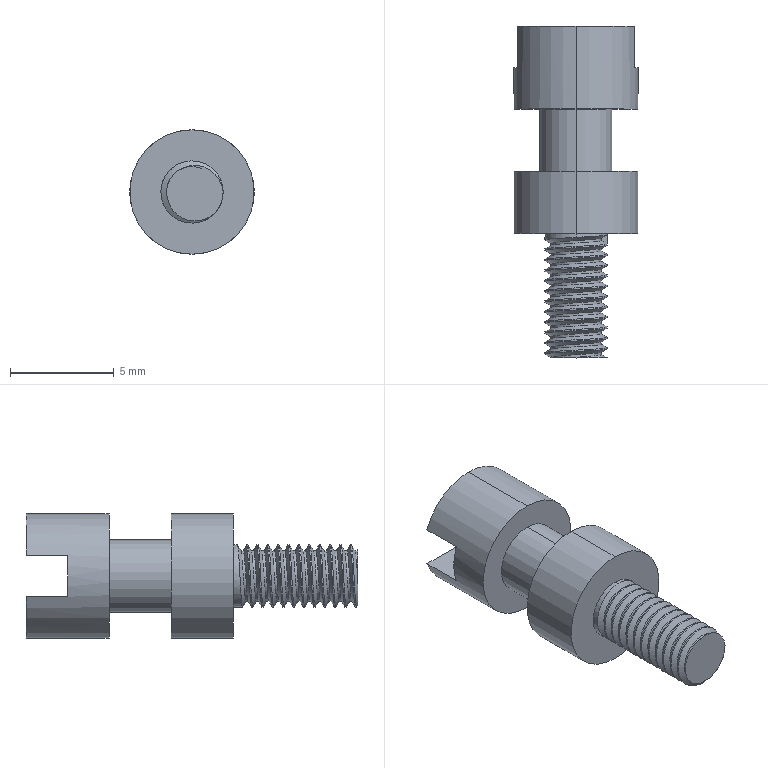Part | NX | features BREP 1 | 1 solid | 43 faces | box 6 x 16 x 6 mm | volume 237.336 mm3 | cylinder 31 | plane 10 | spline 2 | commonest cylinder face diameters 3 x24 6 x4 3.5 x2 2.459 x1